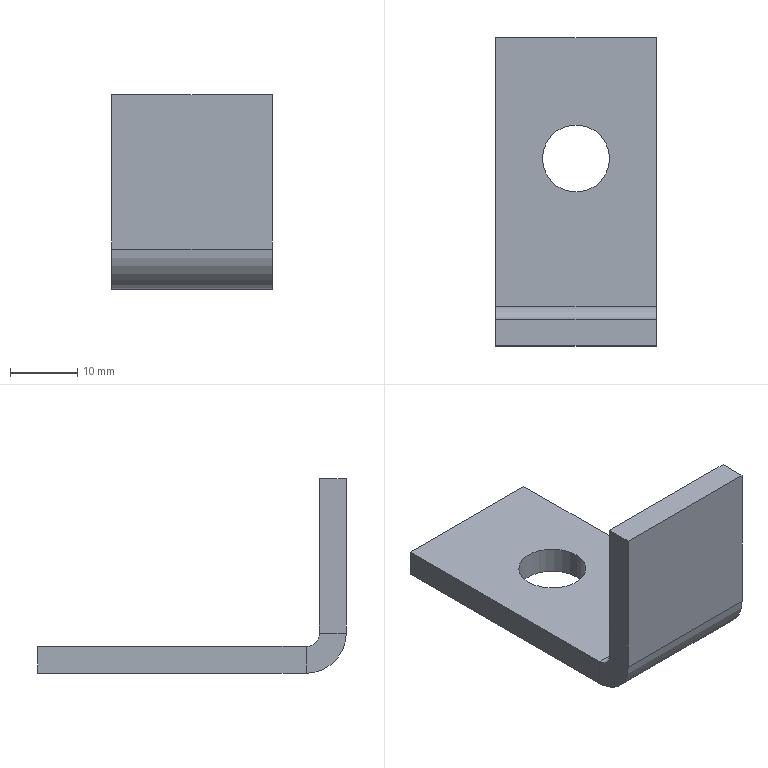Part | STEP file | 001-004-Feeding mechanism cylinder mounting seat | 1 solid | 16 faces | box 24 x 46 x 29 mm | volume 6337 mm3 | plane 12 | cylinder 4 | commonest cylinder face diameters 10 x2 4 x1 12 x1
STEP:
#1=CARTESIAN_POINT('',(0.,0.,0.));
#2=DIRECTION('',(0.,0.,1.));
#3=DIRECTION('',(1.,0.,0.));
#4=AXIS2_PLACEMENT_3D('',#1,#2,#3);
#5=CARTESIAN_POINT('',(5.,2.,-4.));
#6=VERTEX_POINT('',#5);
#7=CARTESIAN_POINT('',(5.,2.,0.));
#8=VERTEX_POINT('',#7);
#9=CARTESIAN_POINT('',(5.,2.,-4.));
#10=DIRECTION('',(0.,0.,1.));
#11=VECTOR('',#10,1.);
#12=LINE('',#9,#11);
#13=CARTESIAN_POINT('',(0.,2.,-4.));
#14=DIRECTION('',(0.,0.,1.));
#15=DIRECTION('',(1.,0.,0.));
#16=AXIS2_PLACEMENT_3D('',#13,#14,#15);
#17=CYLINDRICAL_SURFACE('',#16,5.);
#18=CARTESIAN_POINT('',(6.283,0.));
#19=DIRECTION('',(0.,1.));
#20=VECTOR('',#19,1.);
#21=LINE('',#18,#20);
#22=(GEOMETRIC_REPRESENTATION_CONTEXT(2)PARAMETRIC_REPRESENTATION_CONTEXT()REPRESENTATION_CONTEXT('',''));
#23=DEFINITIONAL_REPRESENTATION('',(#21),#22);
#24=PCURVE('',#17,#23);
#25=CARTESIAN_POINT('',(0.,2.,-4.));
#26=DIRECTION('',(0.,0.,1.));
#27=DIRECTION('',(1.,0.,0.));
#28=AXIS2_PLACEMENT_3D('',#25,#26,#27);
#29=CYLINDRICAL_SURFACE('',#28,5.);
#30=CARTESIAN_POINT('',(0.,0.));
#31=DIRECTION('',(0.,1.));
#32=VECTOR('',#31,1.);
#33=LINE('',#30,#32);
#34=(GEOMETRIC_REPRESENTATION_CONTEXT(2)PARAMETRIC_REPRESENTATION_CONTEXT()REPRESENTATION_CONTEXT('',''));
#35=DEFINITIONAL_REPRESENTATION('',(#33),#34);
#36=PCURVE('',#29,#35);
#37=SURFACE_CURVE('',#12,(#24,#36),.PCURVE_S1.);
#38=EDGE_CURVE('',#6,#8,#37,.T.);
#39=ORIENTED_EDGE('',*,*,#38,.T.);
#40=CARTESIAN_POINT('',(-5.,2.,0.));
#41=VERTEX_POINT('',#40);
#42=CARTESIAN_POINT('',(0.,2.,0.));
#43=DIRECTION('',(0.,0.,1.));
#44=DIRECTION('',(1.,0.,0.));
#45=AXIS2_PLACEMENT_3D('',#42,#43,#44);
#46=CIRCLE('',#45,5.);
#47=CARTESIAN_POINT('',(0.,4.));
#48=DIRECTION('',(1.,0.));
#49=VECTOR('',#48,1.);
#50=LINE('',#47,#49);
#51=(GEOMETRIC_REPRESENTATION_CONTEXT(2)PARAMETRIC_REPRESENTATION_CONTEXT()REPRESENTATION_CONTEXT('',''));
#52=DEFINITIONAL_REPRESENTATION('',(#50),#51);
#53=PCURVE('',#17,#52);
#54=CARTESIAN_POINT('',(0.,0.,0.));
#55=DIRECTION('',(0.,0.,-1.));
#56=DIRECTION('',(-1.,0.,0.));
#57=AXIS2_PLACEMENT_3D('',#54,#55,#56);
#58=PLANE('',#57);
#59=CARTESIAN_POINT('',(-5.,2.));
#60=CARTESIAN_POINT('',(-5.,10.66));
#61=CARTESIAN_POINT('',(2.5,6.33));
#62=CARTESIAN_POINT('',(10.,2.));
#63=CARTESIAN_POINT('',(2.5,-2.33));
#64=CARTESIAN_POINT('',(-5.,-6.66));
#65=CARTESIAN_POINT('',(-5.,2.));
#66=(BOUNDED_CURVE()B_SPLINE_CURVE(2,(#59,#60,#61,#62,#63,#64,#65),.UNSPECIFIED.,.T.,.F.)B_SPLINE_CURVE_WITH_KNOTS((1,2,2,2,2,1),(-2.094,0.,2.094,4.189,6.283,8.378),.UNSPECIFIED.)CURVE()GEOMETRIC_REPRESENTATION_ITEM()RATIONAL_B_SPLINE_CURVE((1.,0.5,1.,0.5,1.,0.5,1.))REPRESENTATION_ITEM(''));
#67=(GEOMETRIC_REPRESENTATION_CONTEXT(2)PARAMETRIC_REPRESENTATION_CONTEXT()REPRESENTATION_CONTEXT('',''));
#68=DEFINITIONAL_REPRESENTATION('',(#66),#67);
#69=PCURVE('',#58,#68);
#70=SURFACE_CURVE('',#46,(#53,#69),.PCURVE_S1.);
#71=EDGE_CURVE('',#41,#8,#70,.T.);
#72=ORIENTED_EDGE('',*,*,#71,.F.);
#73=CARTESIAN_POINT('',(-5.,2.,-4.));
#74=VERTEX_POINT('',#73);
#75=CARTESIAN_POINT('',(-5.,2.,-4.));
#76=DIRECTION('',(0.,0.,1.));
#77=VECTOR('',#76,1.);
#78=LINE('',#75,#77);
#79=CARTESIAN_POINT('',(3.142,0.));
#80=DIRECTION('',(0.,1.));
#81=VECTOR('',#80,1.);
#82=LINE('',#79,#81);
#83=(GEOMETRIC_REPRESENTATION_CONTEXT(2)PARAMETRIC_REPRESENTATION_CONTEXT()REPRESENTATION_CONTEXT('',''));
#84=DEFINITIONAL_REPRESENTATION('',(#82),#83);
#85=PCURVE('',#17,#84);
#86=CARTESIAN_POINT('',(3.142,0.));
#87=DIRECTION('',(0.,1.));
#88=VECTOR('',#87,1.);
#89=LINE('',#86,#88);
#90=(GEOMETRIC_REPRESENTATION_CONTEXT(2)PARAMETRIC_REPRESENTATION_CONTEXT()REPRESENTATION_CONTEXT('',''));
#91=DEFINITIONAL_REPRESENTATION('',(#89),#90);
#92=PCURVE('',#29,#91);
#93=SURFACE_CURVE('',#78,(#85,#92),.PCURVE_S1.);
#94=EDGE_CURVE('',#74,#41,#93,.T.);
#95=ORIENTED_EDGE('',*,*,#94,.F.);
#96=CARTESIAN_POINT('',(0.,2.,-4.));
#97=DIRECTION('',(0.,0.,1.));
#98=DIRECTION('',(1.,0.,0.));
#99=AXIS2_PLACEMENT_3D('',#96,#97,#98);
#100=CIRCLE('',#99,5.);
#101=CARTESIAN_POINT('',(0.,0.));
#102=DIRECTION('',(1.,0.));
#103=VECTOR('',#102,1.);
#104=LINE('',#101,#103);
#105=(GEOMETRIC_REPRESENTATION_CONTEXT(2)PARAMETRIC_REPRESENTATION_CONTEXT()REPRESENTATION_CONTEXT('',''));
#106=DEFINITIONAL_REPRESENTATION('',(#104),#105);
#107=PCURVE('',#17,#106);
#108=CARTESIAN_POINT('',(0.,0.,-4.));
#109=DIRECTION('',(0.,0.,-1.));
#110=DIRECTION('',(-1.,0.,0.));
#111=AXIS2_PLACEMENT_3D('',#108,#109,#110);
#112=PLANE('',#111);
#113=CARTESIAN_POINT('',(-5.,2.));
#114=CARTESIAN_POINT('',(-5.,10.66));
#115=CARTESIAN_POINT('',(2.5,6.33));
#116=CARTESIAN_POINT('',(10.,2.));
#117=CARTESIAN_POINT('',(2.5,-2.33));
#118=CARTESIAN_POINT('',(-5.,-6.66));
#119=CARTESIAN_POINT('',(-5.,2.));
#120=(BOUNDED_CURVE()B_SPLINE_CURVE(2,(#113,#114,#115,#116,#117,#118,#119),.UNSPECIFIED.,.T.,.F.)B_SPLINE_CURVE_WITH_KNOTS((1,2,2,2,2,1),(-2.094,0.,2.094,4.189,6.283,8.378),.UNSPECIFIED.)CURVE()GEOMETRIC_REPRESENTATION_ITEM()RATIONAL_B_SPLINE_CURVE((1.,0.5,1.,0.5,1.,0.5,1.))REPRESENTATION_ITEM(''));
#121=(GEOMETRIC_REPRESENTATION_CONTEXT(2)PARAMETRIC_REPRESENTATION_CONTEXT()REPRESENTATION_CONTEXT('',''));
#122=DEFINITIONAL_REPRESENTATION('',(#120),#121);
#123=PCURVE('',#112,#122);
#124=SURFACE_CURVE('',#100,(#107,#123),.PCURVE_S1.);
#125=EDGE_CURVE('',#74,#6,#124,.T.);
#126=ORIENTED_EDGE('',*,*,#125,.T.);
#127=EDGE_LOOP('',(#39,#72,#95,#126));
#128=FACE_BOUND('',#127,.F.);
#129=ADVANCED_FACE('',(#128),#17,.F.);
#130=CARTESIAN_POINT('',(12.,-20.,0.));
#131=VERTEX_POINT('',#130);
#132=CARTESIAN_POINT('',(12.,20.,0.));
#133=VERTEX_POINT('',#132);
#134=CARTESIAN_POINT('',(12.,-20.,0.));
#135=DIRECTION('',(0.,1.,0.));
#136=VECTOR('',#135,1.);
#137=LINE('',#134,#136);
#138=CARTESIAN_POINT('',(12.,-20.,-4.));
#139=DIRECTION('',(1.,0.,0.));
#140=DIRECTION('',(0.,0.,-1.));
#141=AXIS2_PLACEMENT_3D('',#138,#139,#140);
#142=PLANE('',#141);
#143=CARTESIAN_POINT('',(-4.,0.));
#144=DIRECTION('',(0.,1.));
#145=VECTOR('',#144,1.);
#146=LINE('',#143,#145);
#147=(GEOMETRIC_REPRESENTATION_CONTEXT(2)PARAMETRIC_REPRESENTATION_CONTEXT()REPRESENTATION_CONTEXT('',''));
#148=DEFINITIONAL_REPRESENTATION('',(#146),#147);
#149=PCURVE('',#142,#148);
#150=CARTESIAN_POINT('',(-12.,-20.));
#151=DIRECTION('',(0.,1.));
#152=VECTOR('',#151,1.);
#153=LINE('',#150,#152);
#154=(GEOMETRIC_REPRESENTATION_CONTEXT(2)PARAMETRIC_REPRESENTATION_CONTEXT()REPRESENTATION_CONTEXT('',''));
#155=DEFINITIONAL_REPRESENTATION('',(#153),#154);
#156=PCURVE('',#58,#155);
#157=SURFACE_CURVE('',#137,(#149,#156),.PCURVE_S1.);
#158=EDGE_CURVE('',#131,#133,#157,.T.);
#159=ORIENTED_EDGE('',*,*,#158,.F.);
#160=CARTESIAN_POINT('',(12.,-20.,-4.));
#161=VERTEX_POINT('',#160);
#162=CARTESIAN_POINT('',(12.,-20.,-4.));
#163=DIRECTION('',(0.,0.,1.));
#164=VECTOR('',#163,1.);
#165=LINE('',#162,#164);
#166=CARTESIAN_POINT('',(0.,0.));
#167=DIRECTION('',(-1.,0.));
#168=VECTOR('',#167,1.);
#169=LINE('',#166,#168);
#170=(GEOMETRIC_REPRESENTATION_CONTEXT(2)PARAMETRIC_REPRESENTATION_CONTEXT()REPRESENTATION_CONTEXT('',''));
#171=DEFINITIONAL_REPRESENTATION('',(#169),#170);
#172=PCURVE('',#142,#171);
#173=CARTESIAN_POINT('',(12.,-20.,2.));
#174=DIRECTION('',(-1.,0.,0.));
#175=DIRECTION('',(0.,0.,1.));
#176=AXIS2_PLACEMENT_3D('',#173,#174,#175);
#177=PLANE('',#176);
#178=CARTESIAN_POINT('',(-6.,0.));
#179=DIRECTION('',(1.,0.));
#180=VECTOR('',#179,1.);
#181=LINE('',#178,#180);
#182=(GEOMETRIC_REPRESENTATION_CONTEXT(2)PARAMETRIC_REPRESENTATION_CONTEXT()REPRESENTATION_CONTEXT('',''));
#183=DEFINITIONAL_REPRESENTATION('',(#181),#182);
#184=PCURVE('',#177,#183);
#185=SURFACE_CURVE('',#165,(#172,#184),.PCURVE_S1.);
#186=EDGE_CURVE('',#161,#131,#185,.T.);
#187=ORIENTED_EDGE('',*,*,#186,.F.);
#188=CARTESIAN_POINT('',(12.,20.,-4.));
#189=VERTEX_POINT('',#188);
#190=CARTESIAN_POINT('',(12.,-20.,-4.));
#191=DIRECTION('',(0.,1.,0.));
#192=VECTOR('',#191,1.);
#193=LINE('',#190,#192);
#194=CARTESIAN_POINT('',(0.,0.));
#195=DIRECTION('',(0.,1.));
#196=VECTOR('',#195,1.);
#197=LINE('',#194,#196);
#198=(GEOMETRIC_REPRESENTATION_CONTEXT(2)PARAMETRIC_REPRESENTATION_CONTEXT()REPRESENTATION_CONTEXT('',''));
#199=DEFINITIONAL_REPRESENTATION('',(#197),#198);
#200=PCURVE('',#142,#199);
#201=CARTESIAN_POINT('',(-12.,-20.));
#202=DIRECTION('',(0.,1.));
#203=VECTOR('',#202,1.);
#204=LINE('',#201,#203);
#205=(GEOMETRIC_REPRESENTATION_CONTEXT(2)PARAMETRIC_REPRESENTATION_CONTEXT()REPRESENTATION_CONTEXT('',''));
#206=DEFINITIONAL_REPRESENTATION('',(#204),#205);
#207=PCURVE('',#112,#206);
#208=SURFACE_CURVE('',#193,(#200,#207),.PCURVE_S1.);
#209=EDGE_CURVE('',#161,#189,#208,.T.);
#210=ORIENTED_EDGE('',*,*,#209,.T.);
#211=CARTESIAN_POINT('',(12.,20.,-4.));
#212=DIRECTION('',(0.,0.,1.));
#213=VECTOR('',#212,1.);
#214=LINE('',#211,#213);
#215=CARTESIAN_POINT('',(0.,40.));
#216=DIRECTION('',(-1.,0.));
#217=VECTOR('',#216,1.);
#218=LINE('',#215,#217);
#219=(GEOMETRIC_REPRESENTATION_CONTEXT(2)PARAMETRIC_REPRESENTATION_CONTEXT()REPRESENTATION_CONTEXT('',''));
#220=DEFINITIONAL_REPRESENTATION('',(#218),#219);
#221=PCURVE('',#142,#220);
#222=CARTESIAN_POINT('',(-12.,20.,-4.));
#223=DIRECTION('',(0.,1.,0.));
#224=DIRECTION('',(0.,0.,1.));
#225=AXIS2_PLACEMENT_3D('',#222,#223,#224);
#226=PLANE('',#225);
#227=CARTESIAN_POINT('',(0.,24.));
#228=DIRECTION('',(1.,0.));
#229=VECTOR('',#228,1.);
#230=LINE('',#227,#229);
#231=(GEOMETRIC_REPRESENTATION_CONTEXT(2)PARAMETRIC_REPRESENTATION_CONTEXT()REPRESENTATION_CONTEXT('',''));
#232=DEFINITIONAL_REPRESENTATION('',(#230),#231);
#233=PCURVE('',#226,#232);
#234=SURFACE_CURVE('',#214,(#221,#233),.PCURVE_S1.);
#235=EDGE_CURVE('',#189,#133,#234,.T.);
#236=ORIENTED_EDGE('',*,*,#235,.T.);
#237=EDGE_LOOP('',(#159,#187,#210,#236));
#238=FACE_BOUND('',#237,.T.);
#239=ADVANCED_FACE('',(#238),#142,.T.);
#240=CARTESIAN_POINT('',(-12.,20.,0.));
#241=VERTEX_POINT('',#240);
#242=CARTESIAN_POINT('',(-12.,-20.,0.));
#243=VERTEX_POINT('',#242);
#244=CARTESIAN_POINT('',(-12.,-20.,0.));
#245=DIRECTION('',(0.,-1.,0.));
#246=VECTOR('',#245,1.);
#247=LINE('',#244,#246);
#248=CARTESIAN_POINT('',(-12.,-20.,-4.));
#249=DIRECTION('',(-1.,0.,0.));
#250=DIRECTION('',(0.,0.,1.));
#251=AXIS2_PLACEMENT_3D('',#248,#249,#250);
#252=PLANE('',#251);
#253=CARTESIAN_POINT('',(4.,0.));
#254=DIRECTION('',(0.,-1.));
#255=VECTOR('',#254,1.);
#256=LINE('',#253,#255);
#257=(GEOMETRIC_REPRESENTATION_CONTEXT(2)PARAMETRIC_REPRESENTATION_CONTEXT()REPRESENTATION_CONTEXT('',''));
#258=DEFINITIONAL_REPRESENTATION('',(#256),#257);
#259=PCURVE('',#252,#258);
#260=CARTESIAN_POINT('',(12.,-20.));
#261=DIRECTION('',(0.,-1.));
#262=VECTOR('',#261,1.);
#263=LINE('',#260,#262);
#264=(GEOMETRIC_REPRESENTATION_CONTEXT(2)PARAMETRIC_REPRESENTATION_CONTEXT()REPRESENTATION_CONTEXT('',''));
#265=DEFINITIONAL_REPRESENTATION('',(#263),#264);
#266=PCURVE('',#58,#265);
#267=SURFACE_CURVE('',#247,(#259,#266),.PCURVE_S1.);
#268=EDGE_CURVE('',#241,#243,#267,.T.);
#269=ORIENTED_EDGE('',*,*,#268,.F.);
#270=CARTESIAN_POINT('',(-12.,20.,-4.));
#271=VERTEX_POINT('',#270);
#272=CARTESIAN_POINT('',(-12.,20.,-4.));
#273=DIRECTION('',(0.,0.,1.));
#274=VECTOR('',#273,1.);
#275=LINE('',#272,#274);
#276=CARTESIAN_POINT('',(0.,40.));
#277=DIRECTION('',(1.,0.));
#278=VECTOR('',#277,1.);
#279=LINE('',#276,#278);
#280=(GEOMETRIC_REPRESENTATION_CONTEXT(2)PARAMETRIC_REPRESENTATION_CONTEXT()REPRESENTATION_CONTEXT('',''));
#281=DEFINITIONAL_REPRESENTATION('',(#279),#280);
#282=PCURVE('',#252,#281);
#283=CARTESIAN_POINT('',(0.,0.));
#284=DIRECTION('',(1.,0.));
#285=VECTOR('',#284,1.);
#286=LINE('',#283,#285);
#287=(GEOMETRIC_REPRESENTATION_CONTEXT(2)PARAMETRIC_REPRESENTATION_CONTEXT()REPRESENTATION_CONTEXT('',''));
#288=DEFINITIONAL_REPRESENTATION('',(#286),#287);
#289=PCURVE('',#226,#288);
#290=SURFACE_CURVE('',#275,(#282,#289),.PCURVE_S1.);
#291=EDGE_CURVE('',#271,#241,#290,.T.);
#292=ORIENTED_EDGE('',*,*,#291,.F.);
#293=CARTESIAN_POINT('',(-12.,-20.,-4.));
#294=VERTEX_POINT('',#293);
#295=CARTESIAN_POINT('',(-12.,-20.,-4.));
#296=DIRECTION('',(0.,-1.,0.));
#297=VECTOR('',#296,1.);
#298=LINE('',#295,#297);
#299=CARTESIAN_POINT('',(0.,0.));
#300=DIRECTION('',(0.,-1.));
#301=VECTOR('',#300,1.);
#302=LINE('',#299,#301);
#303=(GEOMETRIC_REPRESENTATION_CONTEXT(2)PARAMETRIC_REPRESENTATION_CONTEXT()REPRESENTATION_CONTEXT('',''));
#304=DEFINITIONAL_REPRESENTATION('',(#302),#303);
#305=PCURVE('',#252,#304);
#306=CARTESIAN_POINT('',(12.,-20.));
#307=DIRECTION('',(0.,-1.));
#308=VECTOR('',#307,1.);
#309=LINE('',#306,#308);
#310=(GEOMETRIC_REPRESENTATION_CONTEXT(2)PARAMETRIC_REPRESENTATION_CONTEXT()REPRESENTATION_CONTEXT('',''));
#311=DEFINITIONAL_REPRESENTATION('',(#309),#310);
#312=PCURVE('',#112,#311);
#313=SURFACE_CURVE('',#298,(#305,#312),.PCURVE_S1.);
#314=EDGE_CURVE('',#271,#294,#313,.T.);
#315=ORIENTED_EDGE('',*,*,#314,.T.);
#316=CARTESIAN_POINT('',(-12.,-20.,-4.));
#317=DIRECTION('',(0.,0.,1.));
#318=VECTOR('',#317,1.);
#319=LINE('',#316,#318);
#320=CARTESIAN_POINT('',(0.,0.));
#321=DIRECTION('',(1.,0.));
#322=VECTOR('',#321,1.);
#323=LINE('',#320,#322);
#324=(GEOMETRIC_REPRESENTATION_CONTEXT(2)PARAMETRIC_REPRESENTATION_CONTEXT()REPRESENTATION_CONTEXT('',''));
#325=DEFINITIONAL_REPRESENTATION('',(#323),#324);
#326=PCURVE('',#252,#325);
#327=CARTESIAN_POINT('',(-12.,-20.,2.));
#328=DIRECTION('',(-1.,0.,0.));
#329=DIRECTION('',(0.,0.,1.));
#330=AXIS2_PLACEMENT_3D('',#327,#328,#329);
#331=PLANE('',#330);
#332=CARTESIAN_POINT('',(-6.,0.));
#333=DIRECTION('',(1.,0.));
#334=VECTOR('',#333,1.);
#335=LINE('',#332,#334);
#336=(GEOMETRIC_REPRESENTATION_CONTEXT(2)PARAMETRIC_REPRESENTATION_CONTEXT()REPRESENTATION_CONTEXT('',''));
#337=DEFINITIONAL_REPRESENTATION('',(#335),#336);
#338=PCURVE('',#331,#337);
#339=SURFACE_CURVE('',#319,(#326,#338),.PCURVE_S1.);
#340=EDGE_CURVE('',#294,#243,#339,.T.);
#341=ORIENTED_EDGE('',*,*,#340,.T.);
#342=EDGE_LOOP('',(#269,#292,#315,#341));
#343=FACE_BOUND('',#342,.T.);
#344=ADVANCED_FACE('',(#343),#252,.T.);
#345=CARTESIAN_POINT('',(-12.,20.,0.));
#346=DIRECTION('',(-1.,0.,0.));
#347=VECTOR('',#346,1.);
#348=LINE('',#345,#347);
#349=CARTESIAN_POINT('',(4.,0.));
#350=DIRECTION('',(0.,-1.));
#351=VECTOR('',#350,1.);
#352=LINE('',#349,#351);
#353=(GEOMETRIC_REPRESENTATION_CONTEXT(2)PARAMETRIC_REPRESENTATION_CONTEXT()REPRESENTATION_CONTEXT('',''));
#354=DEFINITIONAL_REPRESENTATION('',(#352),#353);
#355=PCURVE('',#226,#354);
#356=CARTESIAN_POINT('',(12.,20.));
#357=DIRECTION('',(1.,0.));
#358=VECTOR('',#357,1.);
#359=LINE('',#356,#358);
#360=(GEOMETRIC_REPRESENTATION_CONTEXT(2)PARAMETRIC_REPRESENTATION_CONTEXT()REPRESENTATION_CONTEXT('',''));
#361=DEFINITIONAL_REPRESENTATION('',(#359),#360);
#362=PCURVE('',#58,#361);
#363=SURFACE_CURVE('',#348,(#355,#362),.PCURVE_S1.);
#364=EDGE_CURVE('',#133,#241,#363,.T.);
#365=ORIENTED_EDGE('',*,*,#364,.F.);
#366=ORIENTED_EDGE('',*,*,#235,.F.);
#367=CARTESIAN_POINT('',(-12.,20.,-4.));
#368=DIRECTION('',(-1.,0.,0.));
#369=VECTOR('',#368,1.);
#370=LINE('',#367,#369);
#371=CARTESIAN_POINT('',(0.,0.));
#372=DIRECTION('',(0.,-1.));
#373=VECTOR('',#372,1.);
#374=LINE('',#371,#373);
#375=(GEOMETRIC_REPRESENTATION_CONTEXT(2)PARAMETRIC_REPRESENTATION_CONTEXT()REPRESENTATION_CONTEXT('',''));
#376=DEFINITIONAL_REPRESENTATION('',(#374),#375);
#377=PCURVE('',#226,#376);
#378=CARTESIAN_POINT('',(12.,20.));
#379=DIRECTION('',(1.,0.));
#380=VECTOR('',#379,1.);
#381=LINE('',#378,#380);
#382=(GEOMETRIC_REPRESENTATION_CONTEXT(2)PARAMETRIC_REPRESENTATION_CONTEXT()REPRESENTATION_CONTEXT('',''));
#383=DEFINITIONAL_REPRESENTATION('',(#381),#382);
#384=PCURVE('',#112,#383);
#385=SURFACE_CURVE('',#370,(#377,#384),.PCURVE_S1.);
#386=EDGE_CURVE('',#189,#271,#385,.T.);
#387=ORIENTED_EDGE('',*,*,#386,.T.);
#388=ORIENTED_EDGE('',*,*,#291,.T.);
#389=EDGE_LOOP('',(#365,#366,#387,#388));
#390=FACE_BOUND('',#389,.T.);
#391=ADVANCED_FACE('',(#390),#226,.T.);
#392=CARTESIAN_POINT('',(0.,2.,-4.));
#393=DIRECTION('',(0.,0.,1.));
#394=DIRECTION('',(1.,0.,0.));
#395=AXIS2_PLACEMENT_3D('',#392,#393,#394);
#396=CIRCLE('',#395,5.);
#397=CARTESIAN_POINT('',(-5.,2.));
#398=CARTESIAN_POINT('',(-5.,10.66));
#399=CARTESIAN_POINT('',(2.5,6.33));
#400=CARTESIAN_POINT('',(10.,2.));
#401=CARTESIAN_POINT('',(2.5,-2.33));
#402=CARTESIAN_POINT('',(-5.,-6.66));
#403=CARTESIAN_POINT('',(-5.,2.));
#404=(BOUNDED_CURVE()B_SPLINE_CURVE(2,(#397,#398,#399,#400,#401,#402,#403),.UNSPECIFIED.,.T.,.F.)B_SPLINE_CURVE_WITH_KNOTS((1,2,2,2,2,1),(-2.094,0.,2.094,4.189,6.283,8.378),.UNSPECIFIED.)CURVE()GEOMETRIC_REPRESENTATION_ITEM()RATIONAL_B_SPLINE_CURVE((1.,0.5,1.,0.5,1.,0.5,1.))REPRESENTATION_ITEM(''));
#405=(GEOMETRIC_REPRESENTATION_CONTEXT(2)PARAMETRIC_REPRESENTATION_CONTEXT()REPRESENTATION_CONTEXT('',''));
#406=DEFINITIONAL_REPRESENTATION('',(#404),#405);
#407=PCURVE('',#112,#406);
#408=CARTESIAN_POINT('',(0.,0.));
#409=DIRECTION('',(1.,0.));
#410=VECTOR('',#409,1.);
#411=LINE('',#408,#410);
#412=(GEOMETRIC_REPRESENTATION_CONTEXT(2)PARAMETRIC_REPRESENTATION_CONTEXT()REPRESENTATION_CONTEXT('',''));
#413=DEFINITIONAL_REPRESENTATION('',(#411),#412);
#414=PCURVE('',#29,#413);
#415=SURFACE_CURVE('',#396,(#407,#414),.PCURVE_S1.);
#416=EDGE_CURVE('',#6,#74,#415,.T.);
#417=ORIENTED_EDGE('',*,*,#416,.T.);
#418=ORIENTED_EDGE('',*,*,#125,.T.);
#419=EDGE_LOOP('',(#417,#418));
#420=FACE_BOUND('',#419,.T.);
#421=ORIENTED_EDGE('',*,*,#209,.F.);
#422=CARTESIAN_POINT('',(-12.,-20.,-4.));
#423=DIRECTION('',(1.,0.,0.));
#424=VECTOR('',#423,1.);
#425=LINE('',#422,#424);
#426=CARTESIAN_POINT('',(12.,-20.));
#427=DIRECTION('',(-1.,0.));
#428=VECTOR('',#427,1.);
#429=LINE('',#426,#428);
#430=(GEOMETRIC_REPRESENTATION_CONTEXT(2)PARAMETRIC_REPRESENTATION_CONTEXT()REPRESENTATION_CONTEXT('',''));
#431=DEFINITIONAL_REPRESENTATION('',(#429),#430);
#432=PCURVE('',#112,#431);
#433=CARTESIAN_POINT('',(12.,-20.,2.));
#434=DIRECTION('',(1.,0.,0.));
#435=DIRECTION('',(0.,-1.,0.));
#436=AXIS2_PLACEMENT_3D('',#433,#434,#435);
#437=CYLINDRICAL_SURFACE('',#436,6.);
#438=CARTESIAN_POINT('',(1.571,-24.));
#439=DIRECTION('',(0.,1.));
#440=VECTOR('',#439,1.);
#441=LINE('',#438,#440);
#442=(GEOMETRIC_REPRESENTATION_CONTEXT(2)PARAMETRIC_REPRESENTATION_CONTEXT()REPRESENTATION_CONTEXT('',''));
#443=DEFINITIONAL_REPRESENTATION('',(#441),#442);
#444=PCURVE('',#437,#443);
#445=SURFACE_CURVE('',#425,(#432,#444),.PCURVE_S1.);
#446=EDGE_CURVE('',#294,#161,#445,.T.);
#447=ORIENTED_EDGE('',*,*,#446,.F.);
#448=ORIENTED_EDGE('',*,*,#314,.F.);
#449=ORIENTED_EDGE('',*,*,#386,.F.);
#450=EDGE_LOOP('',(#421,#447,#448,#449));
#451=FACE_BOUND('',#450,.T.);
#452=ADVANCED_FACE('',(#420,#451),#112,.T.);
#453=CARTESIAN_POINT('',(0.,2.,0.));
#454=DIRECTION('',(0.,0.,1.));
#455=DIRECTION('',(1.,0.,0.));
#456=AXIS2_PLACEMENT_3D('',#453,#454,#455);
#457=CIRCLE('',#456,5.);
#458=CARTESIAN_POINT('',(-5.,2.));
#459=CARTESIAN_POINT('',(-5.,10.66));
#460=CARTESIAN_POINT('',(2.5,6.33));
#461=CARTESIAN_POINT('',(10.,2.));
#462=CARTESIAN_POINT('',(2.5,-2.33));
#463=CARTESIAN_POINT('',(-5.,-6.66));
#464=CARTESIAN_POINT('',(-5.,2.));
#465=(BOUNDED_CURVE()B_SPLINE_CURVE(2,(#458,#459,#460,#461,#462,#463,#464),.UNSPECIFIED.,.T.,.F.)B_SPLINE_CURVE_WITH_KNOTS((1,2,2,2,2,1),(-2.094,0.,2.094,4.189,6.283,8.378),.UNSPECIFIED.)CURVE()GEOMETRIC_REPRESENTATION_ITEM()RATIONAL_B_SPLINE_CURVE((1.,0.5,1.,0.5,1.,0.5,1.))REPRESENTATION_ITEM(''));
#466=(GEOMETRIC_REPRESENTATION_CONTEXT(2)PARAMETRIC_REPRESENTATION_CONTEXT()REPRESENTATION_CONTEXT('',''));
#467=DEFINITIONAL_REPRESENTATION('',(#465),#466);
#468=PCURVE('',#58,#467);
#469=CARTESIAN_POINT('',(0.,4.));
#470=DIRECTION('',(1.,0.));
#471=VECTOR('',#470,1.);
#472=LINE('',#469,#471);
#473=(GEOMETRIC_REPRESENTATION_CONTEXT(2)PARAMETRIC_REPRESENTATION_CONTEXT()REPRESENTATION_CONTEXT('',''));
#474=DEFINITIONAL_REPRESENTATION('',(#472),#473);
#475=PCURVE('',#29,#474);
#476=SURFACE_CURVE('',#457,(#468,#475),.PCURVE_S1.);
#477=EDGE_CURVE('',#8,#41,#476,.T.);
#478=ORIENTED_EDGE('',*,*,#477,.F.);
#479=ORIENTED_EDGE('',*,*,#71,.F.);
#480=EDGE_LOOP('',(#478,#479));
#481=FACE_BOUND('',#480,.T.);
#482=ORIENTED_EDGE('',*,*,#158,.T.);
#483=ORIENTED_EDGE('',*,*,#364,.T.);
#484=ORIENTED_EDGE('',*,*,#268,.T.);
#485=CARTESIAN_POINT('',(-12.,-20.,0.));
#486=DIRECTION('',(1.,0.,0.));
#487=VECTOR('',#486,1.);
#488=LINE('',#485,#487);
#489=CARTESIAN_POINT('',(12.,-20.));
#490=DIRECTION('',(-1.,0.));
#491=VECTOR('',#490,1.);
#492=LINE('',#489,#491);
#493=(GEOMETRIC_REPRESENTATION_CONTEXT(2)PARAMETRIC_REPRESENTATION_CONTEXT()REPRESENTATION_CONTEXT('',''));
#494=DEFINITIONAL_REPRESENTATION('',(#492),#493);
#495=PCURVE('',#58,#494);
#496=CARTESIAN_POINT('',(12.,-20.,2.));
#497=DIRECTION('',(1.,0.,0.));
#498=DIRECTION('',(0.,-1.,0.));
#499=AXIS2_PLACEMENT_3D('',#496,#497,#498);
#500=CYLINDRICAL_SURFACE('',#499,2.);
#501=CARTESIAN_POINT('',(1.571,-24.));
#502=DIRECTION('',(0.,1.));
#503=VECTOR('',#502,1.);
#504=LINE('',#501,#503);
#505=(GEOMETRIC_REPRESENTATION_CONTEXT(2)PARAMETRIC_REPRESENTATION_CONTEXT()REPRESENTATION_CONTEXT('',''));
#506=DEFINITIONAL_REPRESENTATION('',(#504),#505);
#507=PCURVE('',#500,#506);
#508=SURFACE_CURVE('',#488,(#495,#507),.PCURVE_S1.);
#509=EDGE_CURVE('',#243,#131,#508,.T.);
#510=ORIENTED_EDGE('',*,*,#509,.T.);
#511=EDGE_LOOP('',(#482,#483,#484,#510));
#512=FACE_BOUND('',#511,.T.);
#513=ADVANCED_FACE('',(#481,#512),#58,.F.);
#514=CARTESIAN_POINT('',(-12.,-22.,2.));
#515=VERTEX_POINT('',#514);
#516=CARTESIAN_POINT('',(-12.,-26.,2.));
#517=VERTEX_POINT('',#516);
#518=CARTESIAN_POINT('',(-12.,-26.,2.));
#519=DIRECTION('',(0.,-1.,0.));
#520=VECTOR('',#519,1.);
#521=LINE('',#518,#520);
#522=CARTESIAN_POINT('',(0.,-6.));
#523=DIRECTION('',(0.,-1.));
#524=VECTOR('',#523,1.);
#525=LINE('',#522,#524);
#526=(GEOMETRIC_REPRESENTATION_CONTEXT(2)PARAMETRIC_REPRESENTATION_CONTEXT()REPRESENTATION_CONTEXT('',''));
#527=DEFINITIONAL_REPRESENTATION('',(#525),#526);
#528=PCURVE('',#331,#527);
#529=CARTESIAN_POINT('',(-12.,-26.,0.));
#530=DIRECTION('',(1.,0.,0.));
#531=DIRECTION('',(0.,0.,-1.));
#532=AXIS2_PLACEMENT_3D('',#529,#530,#531);
#533=PLANE('',#532);
#534=CARTESIAN_POINT('',(-2.,0.));
#535=DIRECTION('',(0.,-1.));
#536=VECTOR('',#535,1.);
#537=LINE('',#534,#536);
#538=(GEOMETRIC_REPRESENTATION_CONTEXT(2)PARAMETRIC_REPRESENTATION_CONTEXT()REPRESENTATION_CONTEXT('',''));
#539=DEFINITIONAL_REPRESENTATION('',(#537),#538);
#540=PCURVE('',#533,#539);
#541=SURFACE_CURVE('',#521,(#528,#540),.PCURVE_S1.);
#542=EDGE_CURVE('',#515,#517,#541,.T.);
#543=ORIENTED_EDGE('',*,*,#542,.F.);
#544=CARTESIAN_POINT('',(-12.,-20.,2.));
#545=DIRECTION('',(-1.,0.,0.));
#546=DIRECTION('',(0.,0.,-1.));
#547=AXIS2_PLACEMENT_3D('',#544,#545,#546);
#548=CIRCLE('',#547,2.);
#549=CARTESIAN_POINT('',(0.,0.));
#550=DIRECTION('',(-1.,0.));
#551=AXIS2_PLACEMENT_2D('',#549,#550);
#552=CIRCLE('',#551,2.);
#553=(GEOMETRIC_REPRESENTATION_CONTEXT(2)PARAMETRIC_REPRESENTATION_CONTEXT()REPRESENTATION_CONTEXT('',''));
#554=DEFINITIONAL_REPRESENTATION('',(#552),#553);
#555=PCURVE('',#331,#554);
#556=CARTESIAN_POINT('',(1.571,-24.));
#557=DIRECTION('',(-1.,0.));
#558=VECTOR('',#557,1.);
#559=LINE('',#556,#558);
#560=(GEOMETRIC_REPRESENTATION_CONTEXT(2)PARAMETRIC_REPRESENTATION_CONTEXT()REPRESENTATION_CONTEXT('',''));
#561=DEFINITIONAL_REPRESENTATION('',(#559),#560);
#562=PCURVE('',#500,#561);
#563=SURFACE_CURVE('',#548,(#555,#562),.PCURVE_S1.);
#564=EDGE_CURVE('',#243,#515,#563,.T.);
#565=ORIENTED_EDGE('',*,*,#564,.F.);
#566=ORIENTED_EDGE('',*,*,#340,.F.);
#567=CARTESIAN_POINT('',(-12.,-20.,2.));
#568=DIRECTION('',(-1.,0.,0.));
#569=DIRECTION('',(0.,0.,-1.));
#570=AXIS2_PLACEMENT_3D('',#567,#568,#569);
#571=CIRCLE('',#570,6.);
#572=CARTESIAN_POINT('',(0.,0.));
#573=DIRECTION('',(-1.,0.));
#574=AXIS2_PLACEMENT_2D('',#572,#573);
#575=CIRCLE('',#574,6.);
#576=(GEOMETRIC_REPRESENTATION_CONTEXT(2)PARAMETRIC_REPRESENTATION_CONTEXT()REPRESENTATION_CONTEXT('',''));
#577=DEFINITIONAL_REPRESENTATION('',(#575),#576);
#578=PCURVE('',#331,#577);
#579=CARTESIAN_POINT('',(1.571,-24.));
#580=DIRECTION('',(-1.,0.));
#581=VECTOR('',#580,1.);
#582=LINE('',#579,#581);
#583=(GEOMETRIC_REPRESENTATION_CONTEXT(2)PARAMETRIC_REPRESENTATION_CONTEXT()REPRESENTATION_CONTEXT('',''));
#584=DEFINITIONAL_REPRESENTATION('',(#582),#583);
#585=PCURVE('',#437,#584);
#586=SURFACE_CURVE('',#571,(#578,#585),.PCURVE_S1.);
#587=EDGE_CURVE('',#294,#517,#586,.T.);
#588=ORIENTED_EDGE('',*,*,#587,.T.);
#589=EDGE_LOOP('',(#543,#565,#566,#588));
#590=FACE_BOUND('',#589,.T.);
#591=ADVANCED_FACE('',(#590),#331,.T.);
#592=CARTESIAN_POINT('',(12.,-22.,2.));
#593=VERTEX_POINT('',#592);
#594=CARTESIAN_POINT('',(12.,-20.,2.));
#595=DIRECTION('',(1.,0.,0.));
#596=DIRECTION('',(0.,0.,-1.));
#597=AXIS2_PLACEMENT_3D('',#594,#595,#596);
#598=CIRCLE('',#597,2.);
#599=CARTESIAN_POINT('',(-2.,0.));
#600=CARTESIAN_POINT('',(-2.,3.464));
#601=CARTESIAN_POINT('',(1.,1.732));
#602=CARTESIAN_POINT('',(4.,0.));
#603=CARTESIAN_POINT('',(1.,-1.732));
#604=CARTESIAN_POINT('',(-2.,-3.464));
#605=CARTESIAN_POINT('',(-2.,0.));
#606=(BOUNDED_CURVE()B_SPLINE_CURVE(2,(#599,#600,#601,#602,#603,#604,#605),.UNSPECIFIED.,.T.,.F.)B_SPLINE_CURVE_WITH_KNOTS((1,2,2,2,2,1),(-2.094,0.,2.094,4.189,6.283,8.378),.UNSPECIFIED.)CURVE()GEOMETRIC_REPRESENTATION_ITEM()RATIONAL_B_SPLINE_CURVE((1.,0.5,1.,0.5,1.,0.5,1.))REPRESENTATION_ITEM(''));
#607=(GEOMETRIC_REPRESENTATION_CONTEXT(2)PARAMETRIC_REPRESENTATION_CONTEXT()REPRESENTATION_CONTEXT('',''));
#608=DEFINITIONAL_REPRESENTATION('',(#606),#607);
#609=PCURVE('',#177,#608);
#610=CARTESIAN_POINT('',(-4.712,0.));
#611=DIRECTION('',(1.,0.));
#612=VECTOR('',#611,1.);
#613=LINE('',#610,#612);
#614=(GEOMETRIC_REPRESENTATION_CONTEXT(2)PARAMETRIC_REPRESENTATION_CONTEXT()REPRESENTATION_CONTEXT('',''));
#615=DEFINITIONAL_REPRESENTATION('',(#613),#614);
#616=PCURVE('',#500,#615);
#617=SURFACE_CURVE('',#598,(#609,#616),.PCURVE_S1.);
#618=EDGE_CURVE('',#593,#131,#617,.T.);
#619=ORIENTED_EDGE('',*,*,#618,.F.);
#620=CARTESIAN_POINT('',(12.,-26.,2.));
#621=VERTEX_POINT('',#620);
#622=CARTESIAN_POINT('',(12.,-22.,2.));
#623=DIRECTION('',(0.,-1.,0.));
#624=VECTOR('',#623,1.);
#625=LINE('',#622,#624);
#626=CARTESIAN_POINT('',(0.,-2.));
#627=DIRECTION('',(0.,-1.));
#628=VECTOR('',#627,1.);
#629=LINE('',#626,#628);
#630=(GEOMETRIC_REPRESENTATION_CONTEXT(2)PARAMETRIC_REPRESENTATION_CONTEXT()REPRESENTATION_CONTEXT('',''));
#631=DEFINITIONAL_REPRESENTATION('',(#629),#630);
#632=PCURVE('',#177,#631);
#633=CARTESIAN_POINT('',(12.,-26.,25.));
#634=DIRECTION('',(-1.,0.,0.));
#635=DIRECTION('',(0.,0.,1.));
#636=AXIS2_PLACEMENT_3D('',#633,#634,#635);
#637=PLANE('',#636);
#638=CARTESIAN_POINT('',(-23.,4.));
#639=DIRECTION('',(0.,-1.));
#640=VECTOR('',#639,1.);
#641=LINE('',#638,#640);
#642=(GEOMETRIC_REPRESENTATION_CONTEXT(2)PARAMETRIC_REPRESENTATION_CONTEXT()REPRESENTATION_CONTEXT('',''));
#643=DEFINITIONAL_REPRESENTATION('',(#641),#642);
#644=PCURVE('',#637,#643);
#645=SURFACE_CURVE('',#625,(#632,#644),.PCURVE_S1.);
#646=EDGE_CURVE('',#593,#621,#645,.T.);
#647=ORIENTED_EDGE('',*,*,#646,.T.);
#648=CARTESIAN_POINT('',(12.,-20.,2.));
#649=DIRECTION('',(1.,0.,0.));
#650=DIRECTION('',(0.,0.,-1.));
#651=AXIS2_PLACEMENT_3D('',#648,#649,#650);
#652=CIRCLE('',#651,6.);
#653=CARTESIAN_POINT('',(-6.,0.));
#654=CARTESIAN_POINT('',(-6.,10.392));
#655=CARTESIAN_POINT('',(3.,5.196));
#656=CARTESIAN_POINT('',(12.,0.));
#657=CARTESIAN_POINT('',(3.,-5.196));
#658=CARTESIAN_POINT('',(-6.,-10.392));
#659=CARTESIAN_POINT('',(-6.,0.));
#660=(BOUNDED_CURVE()B_SPLINE_CURVE(2,(#653,#654,#655,#656,#657,#658,#659),.UNSPECIFIED.,.T.,.F.)B_SPLINE_CURVE_WITH_KNOTS((1,2,2,2,2,1),(-2.094,0.,2.094,4.189,6.283,8.378),.UNSPECIFIED.)CURVE()GEOMETRIC_REPRESENTATION_ITEM()RATIONAL_B_SPLINE_CURVE((1.,0.5,1.,0.5,1.,0.5,1.))REPRESENTATION_ITEM(''));
#661=(GEOMETRIC_REPRESENTATION_CONTEXT(2)PARAMETRIC_REPRESENTATION_CONTEXT()REPRESENTATION_CONTEXT('',''));
#662=DEFINITIONAL_REPRESENTATION('',(#660),#661);
#663=PCURVE('',#177,#662);
#664=CARTESIAN_POINT('',(-4.712,0.));
#665=DIRECTION('',(1.,0.));
#666=VECTOR('',#665,1.);
#667=LINE('',#664,#666);
#668=(GEOMETRIC_REPRESENTATION_CONTEXT(2)PARAMETRIC_REPRESENTATION_CONTEXT()REPRESENTATION_CONTEXT('',''));
#669=DEFINITIONAL_REPRESENTATION('',(#667),#668);
#670=PCURVE('',#437,#669);
#671=SURFACE_CURVE('',#652,(#663,#670),.PCURVE_S1.);
#672=EDGE_CURVE('',#621,#161,#671,.T.);
#673=ORIENTED_EDGE('',*,*,#672,.T.);
#674=ORIENTED_EDGE('',*,*,#186,.T.);
#675=EDGE_LOOP('',(#619,#647,#673,#674));
#676=FACE_BOUND('',#675,.T.);
#677=ADVANCED_FACE('',(#676),#177,.F.);
#678=ORIENTED_EDGE('',*,*,#446,.T.);
#679=ORIENTED_EDGE('',*,*,#672,.F.);
#680=CARTESIAN_POINT('',(-12.,-26.,2.));
#681=DIRECTION('',(-1.,0.,0.));
#682=VECTOR('',#681,1.);
#683=LINE('',#680,#682);
#684=CARTESIAN_POINT('',(0.,-24.));
#685=DIRECTION('',(0.,-1.));
#686=VECTOR('',#685,1.);
#687=LINE('',#684,#686);
#688=(GEOMETRIC_REPRESENTATION_CONTEXT(2)PARAMETRIC_REPRESENTATION_CONTEXT()REPRESENTATION_CONTEXT('',''));
#689=DEFINITIONAL_REPRESENTATION('',(#687),#688);
#690=PCURVE('',#437,#689);
#691=CARTESIAN_POINT('',(0.,-26.,0.));
#692=DIRECTION('',(0.,1.,0.));
#693=DIRECTION('',(0.,0.,1.));
#694=AXIS2_PLACEMENT_3D('',#691,#692,#693);
#695=PLANE('',#694);
#696=CARTESIAN_POINT('',(2.,-12.));
#697=DIRECTION('',(0.,-1.));
#698=VECTOR('',#697,1.);
#699=LINE('',#696,#698);
#700=(GEOMETRIC_REPRESENTATION_CONTEXT(2)PARAMETRIC_REPRESENTATION_CONTEXT()REPRESENTATION_CONTEXT('',''));
#701=DEFINITIONAL_REPRESENTATION('',(#699),#700);
#702=PCURVE('',#695,#701);
#703=SURFACE_CURVE('',#683,(#690,#702),.PCURVE_S1.);
#704=EDGE_CURVE('',#621,#517,#703,.T.);
#705=ORIENTED_EDGE('',*,*,#704,.T.);
#706=ORIENTED_EDGE('',*,*,#587,.F.);
#707=EDGE_LOOP('',(#678,#679,#705,#706));
#708=FACE_BOUND('',#707,.T.);
#709=ADVANCED_FACE('',(#708),#437,.T.);
#710=ORIENTED_EDGE('',*,*,#618,.F.);
#711=CARTESIAN_POINT('',(-12.,-22.,2.));
#712=DIRECTION('',(1.,0.,0.));
#713=VECTOR('',#712,1.);
#714=LINE('',#711,#713);
#715=CARTESIAN_POINT('',(0.,-24.));
#716=DIRECTION('',(0.,1.));
#717=VECTOR('',#716,1.);
#718=LINE('',#715,#717);
#719=(GEOMETRIC_REPRESENTATION_CONTEXT(2)PARAMETRIC_REPRESENTATION_CONTEXT()REPRESENTATION_CONTEXT('',''));
#720=DEFINITIONAL_REPRESENTATION('',(#718),#719);
#721=PCURVE('',#500,#720);
#722=CARTESIAN_POINT('',(0.,-22.,0.));
#723=DIRECTION('',(0.,1.,0.));
#724=DIRECTION('',(0.,0.,1.));
#725=AXIS2_PLACEMENT_3D('',#722,#723,#724);
#726=PLANE('',#725);
#727=CARTESIAN_POINT('',(2.,-12.));
#728=DIRECTION('',(0.,1.));
#729=VECTOR('',#728,1.);
#730=LINE('',#727,#729);
#731=(GEOMETRIC_REPRESENTATION_CONTEXT(2)PARAMETRIC_REPRESENTATION_CONTEXT()REPRESENTATION_CONTEXT('',''));
#732=DEFINITIONAL_REPRESENTATION('',(#730),#731);
#733=PCURVE('',#726,#732);
#734=SURFACE_CURVE('',#714,(#721,#733),.PCURVE_S1.);
#735=EDGE_CURVE('',#515,#593,#734,.T.);
#736=ORIENTED_EDGE('',*,*,#735,.F.);
#737=ORIENTED_EDGE('',*,*,#564,.F.);
#738=ORIENTED_EDGE('',*,*,#509,.T.);
#739=EDGE_LOOP('',(#710,#736,#737,#738));
#740=FACE_BOUND('',#739,.F.);
#741=ADVANCED_FACE('',(#740),#500,.F.);
#742=ORIENTED_EDGE('',*,*,#542,.T.);
#743=CARTESIAN_POINT('',(-12.,-26.,25.));
#744=VERTEX_POINT('',#743);
#745=CARTESIAN_POINT('',(-12.,-26.,0.));
#746=DIRECTION('',(0.,0.,-1.));
#747=VECTOR('',#746,1.);
#748=LINE('',#745,#747);
#749=CARTESIAN_POINT('',(0.,0.));
#750=DIRECTION('',(1.,0.));
#751=VECTOR('',#750,1.);
#752=LINE('',#749,#751);
#753=(GEOMETRIC_REPRESENTATION_CONTEXT(2)PARAMETRIC_REPRESENTATION_CONTEXT()REPRESENTATION_CONTEXT('',''));
#754=DEFINITIONAL_REPRESENTATION('',(#752),#753);
#755=PCURVE('',#533,#754);
#756=CARTESIAN_POINT('',(0.,-12.));
#757=DIRECTION('',(-1.,0.));
#758=VECTOR('',#757,1.);
#759=LINE('',#756,#758);
#760=(GEOMETRIC_REPRESENTATION_CONTEXT(2)PARAMETRIC_REPRESENTATION_CONTEXT()REPRESENTATION_CONTEXT('',''));
#761=DEFINITIONAL_REPRESENTATION('',(#759),#760);
#762=PCURVE('',#695,#761);
#763=SURFACE_CURVE('',#748,(#755,#762),.PCURVE_S1.);
#764=EDGE_CURVE('',#744,#517,#763,.T.);
#765=ORIENTED_EDGE('',*,*,#764,.F.);
#766=CARTESIAN_POINT('',(-12.,-22.,25.));
#767=VERTEX_POINT('',#766);
#768=CARTESIAN_POINT('',(-12.,-26.,25.));
#769=DIRECTION('',(0.,1.,0.));
#770=VECTOR('',#769,1.);
#771=LINE('',#768,#770);
#772=CARTESIAN_POINT('',(-25.,0.));
#773=DIRECTION('',(0.,1.));
#774=VECTOR('',#773,1.);
#775=LINE('',#772,#774);
#776=(GEOMETRIC_REPRESENTATION_CONTEXT(2)PARAMETRIC_REPRESENTATION_CONTEXT()REPRESENTATION_CONTEXT('',''));
#777=DEFINITIONAL_REPRESENTATION('',(#775),#776);
#778=PCURVE('',#533,#777);
#779=CARTESIAN_POINT('',(-12.,-26.,25.));
#780=DIRECTION('',(0.,0.,-1.));
#781=DIRECTION('',(0.,1.,0.));
#782=AXIS2_PLACEMENT_3D('',#779,#780,#781);
#783=PLANE('',#782);
#784=CARTESIAN_POINT('',(0.,0.));
#785=DIRECTION('',(1.,0.));
#786=VECTOR('',#785,1.);
#787=LINE('',#784,#786);
#788=(GEOMETRIC_REPRESENTATION_CONTEXT(2)PARAMETRIC_REPRESENTATION_CONTEXT()REPRESENTATION_CONTEXT('',''));
#789=DEFINITIONAL_REPRESENTATION('',(#787),#788);
#790=PCURVE('',#783,#789);
#791=SURFACE_CURVE('',#771,(#778,#790),.PCURVE_S1.);
#792=EDGE_CURVE('',#744,#767,#791,.T.);
#793=ORIENTED_EDGE('',*,*,#792,.T.);
#794=CARTESIAN_POINT('',(-12.,-22.,0.));
#795=DIRECTION('',(0.,0.,-1.));
#796=VECTOR('',#795,1.);
#797=LINE('',#794,#796);
#798=CARTESIAN_POINT('',(0.,4.));
#799=DIRECTION('',(1.,0.));
#800=VECTOR('',#799,1.);
#801=LINE('',#798,#800);
#802=(GEOMETRIC_REPRESENTATION_CONTEXT(2)PARAMETRIC_REPRESENTATION_CONTEXT()REPRESENTATION_CONTEXT('',''));
#803=DEFINITIONAL_REPRESENTATION('',(#801),#802);
#804=PCURVE('',#533,#803);
#805=CARTESIAN_POINT('',(0.,-12.));
#806=DIRECTION('',(-1.,0.));
#807=VECTOR('',#806,1.);
#808=LINE('',#805,#807);
#809=(GEOMETRIC_REPRESENTATION_CONTEXT(2)PARAMETRIC_REPRESENTATION_CONTEXT()REPRESENTATION_CONTEXT('',''));
#810=DEFINITIONAL_REPRESENTATION('',(#808),#809);
#811=PCURVE('',#726,#810);
#812=SURFACE_CURVE('',#797,(#804,#811),.PCURVE_S1.);
#813=EDGE_CURVE('',#767,#515,#812,.T.);
#814=ORIENTED_EDGE('',*,*,#813,.T.);
#815=EDGE_LOOP('',(#742,#765,#793,#814));
#816=FACE_BOUND('',#815,.T.);
#817=ADVANCED_FACE('',(#816),#533,.F.);
#818=ORIENTED_EDGE('',*,*,#646,.F.);
#819=CARTESIAN_POINT('',(12.,-22.,25.));
#820=VERTEX_POINT('',#819);
#821=CARTESIAN_POINT('',(12.,-22.,25.));
#822=DIRECTION('',(0.,0.,1.));
#823=VECTOR('',#822,1.);
#824=LINE('',#821,#823);
#825=CARTESIAN_POINT('',(0.,4.));
#826=DIRECTION('',(1.,0.));
#827=VECTOR('',#826,1.);
#828=LINE('',#825,#827);
#829=(GEOMETRIC_REPRESENTATION_CONTEXT(2)PARAMETRIC_REPRESENTATION_CONTEXT()REPRESENTATION_CONTEXT('',''));
#830=DEFINITIONAL_REPRESENTATION('',(#828),#829);
#831=PCURVE('',#637,#830);
#832=CARTESIAN_POINT('',(25.,12.));
#833=DIRECTION('',(1.,0.));
#834=VECTOR('',#833,1.);
#835=LINE('',#832,#834);
#836=(GEOMETRIC_REPRESENTATION_CONTEXT(2)PARAMETRIC_REPRESENTATION_CONTEXT()REPRESENTATION_CONTEXT('',''));
#837=DEFINITIONAL_REPRESENTATION('',(#835),#836);
#838=PCURVE('',#726,#837);
#839=SURFACE_CURVE('',#824,(#831,#838),.PCURVE_S1.);
#840=EDGE_CURVE('',#593,#820,#839,.T.);
#841=ORIENTED_EDGE('',*,*,#840,.T.);
#842=CARTESIAN_POINT('',(12.,-26.,25.));
#843=VERTEX_POINT('',#842);
#844=CARTESIAN_POINT('',(12.,-26.,25.));
#845=DIRECTION('',(0.,1.,0.));
#846=VECTOR('',#845,1.);
#847=LINE('',#844,#846);
#848=CARTESIAN_POINT('',(0.,0.));
#849=DIRECTION('',(0.,1.));
#850=VECTOR('',#849,1.);
#851=LINE('',#848,#850);
#852=(GEOMETRIC_REPRESENTATION_CONTEXT(2)PARAMETRIC_REPRESENTATION_CONTEXT()REPRESENTATION_CONTEXT('',''));
#853=DEFINITIONAL_REPRESENTATION('',(#851),#852);
#854=PCURVE('',#637,#853);
#855=CARTESIAN_POINT('',(0.,24.));
#856=DIRECTION('',(1.,0.));
#857=VECTOR('',#856,1.);
#858=LINE('',#855,#857);
#859=(GEOMETRIC_REPRESENTATION_CONTEXT(2)PARAMETRIC_REPRESENTATION_CONTEXT()REPRESENTATION_CONTEXT('',''));
#860=DEFINITIONAL_REPRESENTATION('',(#858),#859);
#861=PCURVE('',#783,#860);
#862=SURFACE_CURVE('',#847,(#854,#861),.PCURVE_S1.);
#863=EDGE_CURVE('',#843,#820,#862,.T.);
#864=ORIENTED_EDGE('',*,*,#863,.F.);
#865=CARTESIAN_POINT('',(12.,-26.,0.));
#866=DIRECTION('',(0.,0.,1.));
#867=VECTOR('',#866,1.);
#868=LINE('',#865,#867);
#869=CARTESIAN_POINT('',(-25.,0.));
#870=DIRECTION('',(1.,0.));
#871=VECTOR('',#870,1.);
#872=LINE('',#869,#871);
#873=(GEOMETRIC_REPRESENTATION_CONTEXT(2)PARAMETRIC_REPRESENTATION_CONTEXT()REPRESENTATION_CONTEXT('',''));
#874=DEFINITIONAL_REPRESENTATION('',(#872),#873);
#875=PCURVE('',#637,#874);
#876=CARTESIAN_POINT('',(0.,12.));
#877=DIRECTION('',(1.,0.));
#878=VECTOR('',#877,1.);
#879=LINE('',#876,#878);
#880=(GEOMETRIC_REPRESENTATION_CONTEXT(2)PARAMETRIC_REPRESENTATION_CONTEXT()REPRESENTATION_CONTEXT('',''));
#881=DEFINITIONAL_REPRESENTATION('',(#879),#880);
#882=PCURVE('',#695,#881);
#883=SURFACE_CURVE('',#868,(#875,#882),.PCURVE_S1.);
#884=EDGE_CURVE('',#621,#843,#883,.T.);
#885=ORIENTED_EDGE('',*,*,#884,.F.);
#886=EDGE_LOOP('',(#818,#841,#864,#885));
#887=FACE_BOUND('',#886,.T.);
#888=ADVANCED_FACE('',(#887),#637,.F.);
#889=ORIENTED_EDGE('',*,*,#704,.F.);
#890=ORIENTED_EDGE('',*,*,#884,.T.);
#891=CARTESIAN_POINT('',(0.,-26.,25.));
#892=DIRECTION('',(-1.,0.,0.));
#893=VECTOR('',#892,1.);
#894=LINE('',#891,#893);
#895=CARTESIAN_POINT('',(25.,0.));
#896=DIRECTION('',(0.,-1.));
#897=VECTOR('',#896,1.);
#898=LINE('',#895,#897);
#899=(GEOMETRIC_REPRESENTATION_CONTEXT(2)PARAMETRIC_REPRESENTATION_CONTEXT()REPRESENTATION_CONTEXT('',''));
#900=DEFINITIONAL_REPRESENTATION('',(#898),#899);
#901=PCURVE('',#695,#900);
#902=CARTESIAN_POINT('',(0.,12.));
#903=DIRECTION('',(0.,-1.));
#904=VECTOR('',#903,1.);
#905=LINE('',#902,#904);
#906=(GEOMETRIC_REPRESENTATION_CONTEXT(2)PARAMETRIC_REPRESENTATION_CONTEXT()REPRESENTATION_CONTEXT('',''));
#907=DEFINITIONAL_REPRESENTATION('',(#905),#906);
#908=PCURVE('',#783,#907);
#909=SURFACE_CURVE('',#894,(#901,#908),.PCURVE_S1.);
#910=EDGE_CURVE('',#843,#744,#909,.T.);
#911=ORIENTED_EDGE('',*,*,#910,.T.);
#912=ORIENTED_EDGE('',*,*,#764,.T.);
#913=EDGE_LOOP('',(#889,#890,#911,#912));
#914=FACE_BOUND('',#913,.T.);
#915=ADVANCED_FACE('',(#914),#695,.F.);
#916=ORIENTED_EDGE('',*,*,#840,.F.);
#917=ORIENTED_EDGE('',*,*,#735,.F.);
#918=ORIENTED_EDGE('',*,*,#813,.F.);
#919=CARTESIAN_POINT('',(-12.,-22.,25.));
#920=DIRECTION('',(-1.,0.,0.));
#921=VECTOR('',#920,1.);
#922=LINE('',#919,#921);
#923=CARTESIAN_POINT('',(25.,-12.));
#924=DIRECTION('',(0.,-1.));
#925=VECTOR('',#924,1.);
#926=LINE('',#923,#925);
#927=(GEOMETRIC_REPRESENTATION_CONTEXT(2)PARAMETRIC_REPRESENTATION_CONTEXT()REPRESENTATION_CONTEXT('',''));
#928=DEFINITIONAL_REPRESENTATION('',(#926),#927);
#929=PCURVE('',#726,#928);
#930=CARTESIAN_POINT('',(4.,0.));
#931=DIRECTION('',(0.,-1.));
#932=VECTOR('',#931,1.);
#933=LINE('',#930,#932);
#934=(GEOMETRIC_REPRESENTATION_CONTEXT(2)PARAMETRIC_REPRESENTATION_CONTEXT()REPRESENTATION_CONTEXT('',''));
#935=DEFINITIONAL_REPRESENTATION('',(#933),#934);
#936=PCURVE('',#783,#935);
#937=SURFACE_CURVE('',#922,(#929,#936),.PCURVE_S1.);
#938=EDGE_CURVE('',#820,#767,#937,.T.);
#939=ORIENTED_EDGE('',*,*,#938,.F.);
#940=EDGE_LOOP('',(#916,#917,#918,#939));
#941=FACE_BOUND('',#940,.T.);
#942=ADVANCED_FACE('',(#941),#726,.T.);
#943=ORIENTED_EDGE('',*,*,#938,.T.);
#944=ORIENTED_EDGE('',*,*,#792,.F.);
#945=ORIENTED_EDGE('',*,*,#910,.F.);
#946=ORIENTED_EDGE('',*,*,#863,.T.);
#947=EDGE_LOOP('',(#943,#944,#945,#946));
#948=FACE_BOUND('',#947,.T.);
#949=ADVANCED_FACE('',(#948),#783,.F.);
#950=ORIENTED_EDGE('',*,*,#477,.F.);
#951=ORIENTED_EDGE('',*,*,#38,.F.);
#952=ORIENTED_EDGE('',*,*,#416,.T.);
#953=ORIENTED_EDGE('',*,*,#94,.T.);
#954=EDGE_LOOP('',(#950,#951,#952,#953));
#955=FACE_BOUND('',#954,.F.);
#956=ADVANCED_FACE('',(#955),#29,.F.);
#957=CLOSED_SHELL('',(#129,#239,#344,#391,#452,#513,#591,#677,#709,#741,#817,#888,#915,#942,#949,#956));
#958=MANIFOLD_SOLID_BREP('',#957);
#959=(LENGTH_UNIT()NAMED_UNIT(*)SI_UNIT(.MILLI.,.METRE.));
#960=UNCERTAINTY_MEASURE_WITH_UNIT(LENGTH_MEASURE(0.0000001),#959,'','');
#961=(NAMED_UNIT(*)PLANE_ANGLE_UNIT()SI_UNIT($,.RADIAN.));
#962=(NAMED_UNIT(*)SI_UNIT($,.STERADIAN.)SOLID_ANGLE_UNIT());
#963=(GEOMETRIC_REPRESENTATION_CONTEXT(3)GLOBAL_UNCERTAINTY_ASSIGNED_CONTEXT((#960))GLOBAL_UNIT_ASSIGNED_CONTEXT((#959,#961,#962))REPRESENTATION_CONTEXT('',''));
#964=ADVANCED_BREP_SHAPE_REPRESENTATION('',(#4,#958),#963);